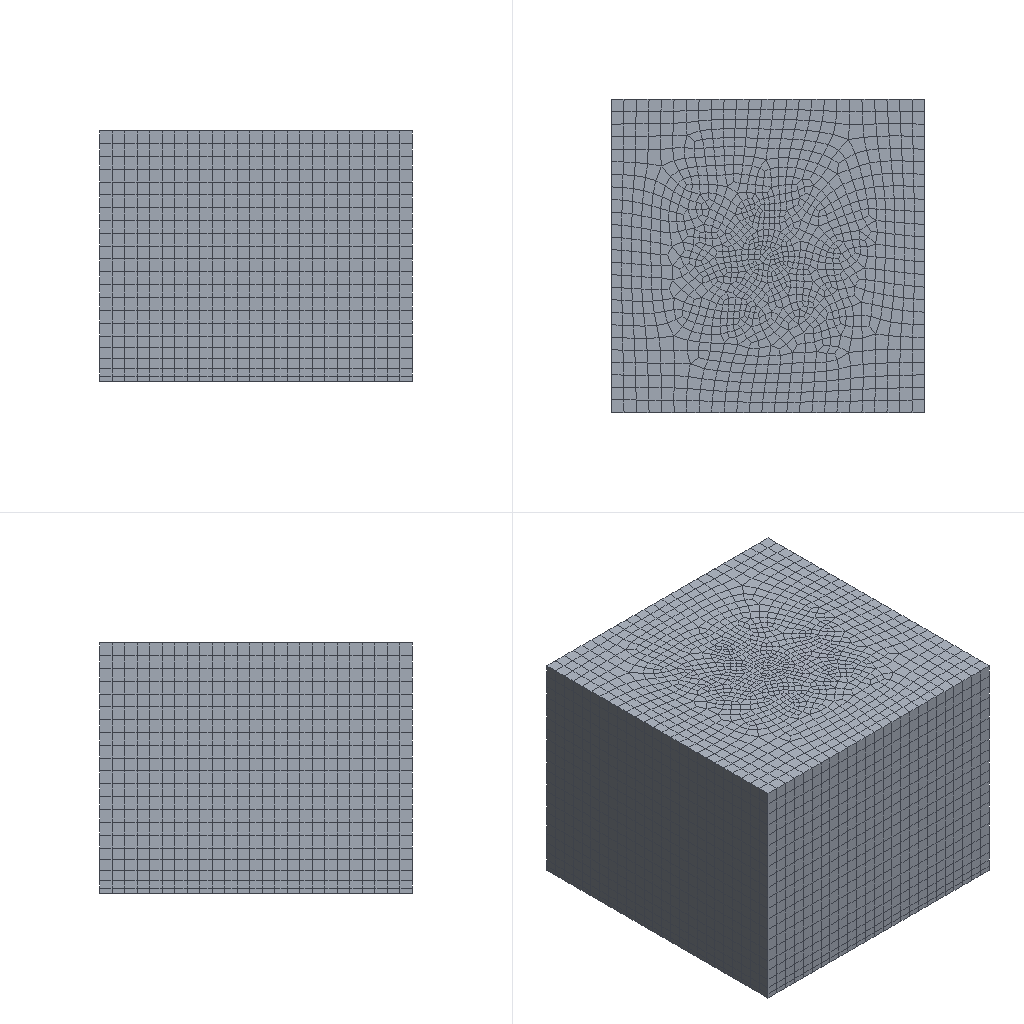Simulation study | abaqus
Set-up summary:
category,name,step,type,value,unit,region
solver,abaqus
solver,version,,,Abaqus/Standard 3DEXPERIENCE R2017x
units,not stated in the deck,,not stated
analysis,deck,,coupled temperature-displacement,coupled temperature-displacement
load_step,Step-1,Step-1,coupled temperature-displacement
load_step,requested,,,1
mesh,nodes,,,27236
mesh,elements,,,24927
element_type,C3D8RT,,solid,24927
load,load commands in deck,,count,2
bc,support commands in deck,,count,7
material,L1,,in results
material,L2,,in results
material,L3,,in results
material,L4,,in results
material,L5,,in results
material,L6,,in results
check,setup vs results,,match,"per instance, exact: element labels, types and connectivity; labels of the nodes the elements use; coordinates of those nodes at SINGLE_PRECISION in 1 of 1 instance(s)"
Abaqus input file, long lists of numbers shortened:
*Heading
** Job name: Job-1 Model name: Model-1
** Generated by: Abaqus/CAE 2017
*Preprint, echo=NO, model=NO, history=NO, contact=NO
**
** PARTS
**
*Part, name=Part-1
*Node
      1,   1388.619,  -1088.278,           0.
      2,           0.,           0.,           0.
** (27234 more lines like these left out)
*Element, type=C3D8RT
   1,  790,   38,   37,  803, 1928, 1908, 1907, 1941
   2,  805,   40,   39,  804, 1943, 1910, 1909, 1942
** (24925 more lines like these left out)
*Nset, nset=Set-6
    1,    2,    3,    4,    5,    6,    7,    8,    9,   30,   31,   32,   33,   34,   35,   36
   37,   38,   39,   40,   41,   42,   43,   44,   45,   46,   47,   48,   49,   50,   51,   52
** (153 more lines like these left out)
*Elset, elset=Set-6, generate
    1,  1187,     1
*Nset, nset=Set-7
    6,    7,    8,    9,   10,   11,   12,   13,  153,  154,  155,  156,  157,  158,  159,  160
  161,  162,  163,  164,  165,  166,  167,  168,  169,  170,  171,  172,  173,  174,  175,  176
** (153 more lines like these left out)
*Elset, elset=Set-7, generate
 1188,  2374,     1
*Nset, nset=Set-8
   10,   11,   12,   13,   14,   15,   16,   17,  249,  250,  251,  252,  253,  254,  255,  256
  257,  258,  259,  260,  261,  262,  263,  264,  265,  266,  267,  268,  269,  270,  271,  272
** (153 more lines like these left out)
*Elset, elset=Set-8, generate
 2375,  3561,     1
*Nset, nset=Set-9
    14,    15,    16,    17,    18,    19,    20,    21,   345,   346,   347,   348,   349,   350,   351,   352
   353,   354,   355,   356,   357,   358,   359,   360,   361,   362,   363,   364,   365,   366,   367,   368
** (231 more lines like these left out)
*Elset, elset=Set-9, generate
 3562,  5935,     1
*Nset, nset=Set-10
    18,    19,    20,    21,    22,    23,    24,    25,   445,   446,   447,   448,   449,   450,   451,   452
   453,   454,   455,   456,   457,   458,   459,   460,   461,   462,   463,   464,   465,   466,   467,   468
** (308 more lines like these left out)
*Elset, elset=Set-10, generate
 5936,  9496,     1
*Nset, nset=Set-11
    22,    23,    24,    25,    26,    27,    28,    29,   549,   550,   551,   552,   553,   554,   555,   556
   557,   558,   559,   560,   561,   562,   563,   564,   565,   566,   567,   568,   569,   570,   571,   572
** (1082 more lines like these left out)
*Elset, elset=Set-11, generate
  9497,  24927,      1
** Section: l1
*Solid Section, elset=Set-6, material=l1
,
** Section: l2
*Solid Section, elset=Set-7, material=l2
,
** Section: l3
*Solid Section, elset=Set-8, material=l3
,
** Section: l4
*Solid Section, elset=Set-9, material=l4
,
** Section: l5
*Solid Section, elset=Set-10, material=l5
,
** Section: l6
*Solid Section, elset=Set-11, material=l6
,
*End Part
**
**
** ASSEMBLY
**
*Assembly, name=Assembly
**
*Instance, name=Part-1-1, part=Part-1
*End Instance
**
*Nset, nset=Set-1, instance=Part-1-1, generate
     1,  27236,      1
*Elset, elset=Set-1, instance=Part-1-1, generate
     1,  24927,      1
*Nset, nset=Set-2, instance=Part-1-1
     1,     2,     3,     4,     5,     6,     7,     8,     9,    10,    11,    12,    13,    14,    15,    16
    17,    18,    19,    20,    21,    22,    23,    24,    25,    26,    27,    28,    29,    30,    31,    32
** (278 more lines like these left out)
*Elset, elset=Set-2, instance=Part-1-1
     1,     2,     3,     4,     5,     6,     7,     8,     9,    10,    11,    12,    13,    14,    15,    16
    17,    18,    19,    20,    21,    22,    23,    24,    25,    26,    27,    28,    29,    30,    31,    32
** (261 more lines like these left out)
*Nset, nset=Set-3, instance=Part-1-1
    22,    23,    24,    25,    26,    27,    28,    29,   549,   550,   551,   552,   553,   554,   555,   556
   557,   558,   559,   560,   561,   562,   563,   564,   565,   566,   567,   568,   569,   570,   571,   572
** (86 more lines like these left out)
*Elset, elset=Set-3, instance=Part-1-1
  9598,  9602,  9603,  9605,  9607,  9613,  9618,  9620,  9621,  9622,  9623,  9624,  9625,  9627,  9628,  9632
  9636,  9637,  9638,  9639,  9640,  9641,  9643,  9644,  9651,  9656,  9657,  9658,  9659,  9660,  9661,  9665
** (76 more lines like these left out)
*Elset, elset=_Surf-1_S1, internal, instance=Part-1-1, generate
  1,  90,   1
*Surface, type=ELEMENT, name=Surf-1
_Surf-1_S1, S1
*End Assembly
*Amplitude, name=Amp-1
             0.,             20.,          43200.,             20.,          44000.,            -20.,          86400.,            -20.
         87000.,             20.,         129600.,             20.,         130000.,            -20.,         172800.,            -20.
        173000.,             20.,         216000.,             20.,         217000.,            -20.,         259200.,            -20.
        260000.,             20.,         302400.,             20.,         303000.,            -20.,         345600.,            -20.
        346000.,             20.,         388800.,             20.,         389000.,            -20.,         432000.,            -20.
        433000.,             20.,         475200.,             20.,         476000.,            -20.,         518400.,            -20.
**
** MATERIALS
**
*Material, name=l1
*Conductivity
820.,
*Density
 2.4e-09,
*Elastic, dependencies=2
1067., 0.3, ,  1.,  1.
*Expansion
 -0.00045,
*Specific Heat
 1.25e+06,
*User Defined Field
*Material, name=l2
*Conductivity
820.,
*Density
 2.4e-09,
*Elastic, dependencies=2
1100., 0.35, ,   1.,   1.
*Expansion
 -0.00045,
*Specific Heat
 1.25e+06,
*User Defined Field
*Material, name=l3
*Conductivity
820.,
*Density
 2.4e-09,
*Elastic, dependencies=2
900., 0.35, ,   1.,   1.
*Expansion
 -0.00045,
*Specific Heat
 1.25e+06,
*User Defined Field
*Material, name=l4
*Conductivity
3.,
*Density
 2.4e-09,
*Elastic
1500., 0.2
*Specific Heat
 9e+08,
*Material, name=l5
*Conductivity
3.,
*Density
 2.4e-09,
*Elastic
1500., 0.2
*Specific Heat
 9e+08,
*Material, name=l6
*Conductivity
3.,
*Density
 2.4e-09,
*Elastic
40., 0.35
*Specific Heat
 9e+08,
** ----------------------------------------------------------------
**
** STEP: Step-1
**
*Step, name=Step-1, nlgeom=YES, inc=100000
*Coupled Temperature-displacement, creep=none, deltmx=1e+09, stabilize=0.0002, allsdtol=0.05, continue=NO
1., 51840., 0.05184, 2000.
**
** BOUNDARY CONDITIONS
**
** Name: BC-1 Type: 温度
*Boundary, amplitude=Amp-1
Set-2, 11, 11, 1.
** Name: BC-2 Type: 位移/转角
*Boundary
Set-3, 1, 1
Set-3, 2, 2
Set-3, 3, 3
Set-3, 4, 4
Set-3, 5, 5
Set-3, 6, 6
**
** LOADS
**
** Name: Load-1   Type: Pressure
*Dsload
Surf-1, P, 0.7
**
** OUTPUT REQUESTS
**
*Restart, write, frequency=0
**
** FIELD OUTPUT: F-Output-1
**
*Output, field
*Node Output
CF, NT, RF, RFL, RM, RT, TF, U
V
*Element Output, directions=YES
E, HFL, LE, MISES, MISESMAX, MISESONLY, PE, PEEQ, PEEQT, PEMAG, S, SF, SSAVG, TEMP, TSHR, VEEQ
*Contact Output
CDISP, CSTRESS
*Radiation Output
FTEMP,
**
** HISTORY OUTPUT: H-Output-1
**
*Output, history, variable=PRESELECT
*End Step
Results summary:
result,step,,completed,increments=44 time=51840.0/51840.0
result,analysis,,,"coupled temperature-displacement, steady state"
result,last_loadstep,,,1
result,primary field,,,"U, NT11"
result,reaction total,,FX,0.6734,model units
result,reaction total,,FY,-2.032,model units
result,reaction total,,FZ,-100009.124,model units